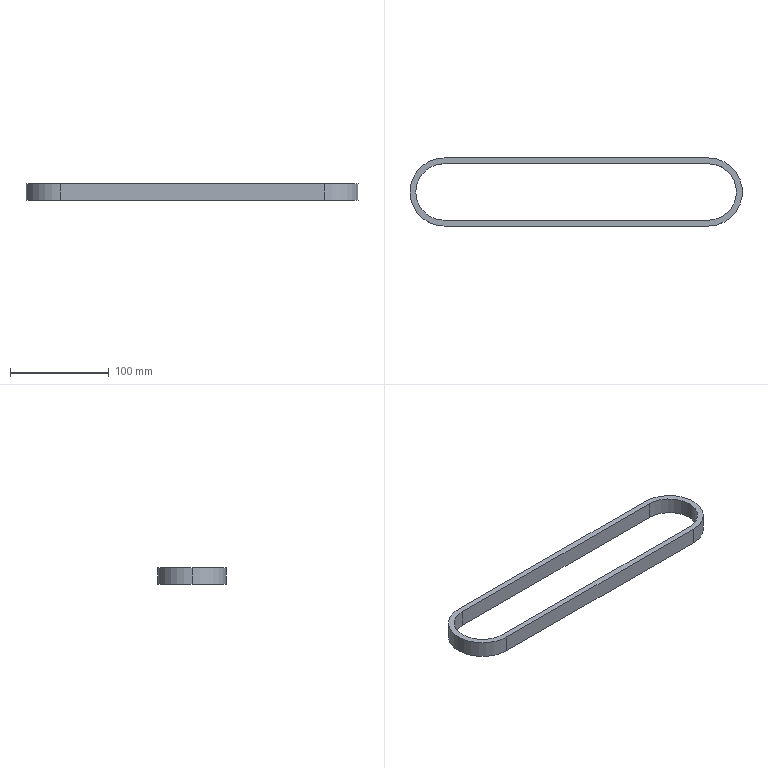Part | SolidWorks | features BaseBody 1 | 1 solid | 12 faces | box 335.87 x 68.87 x 17 mm | volume 73402 mm3 | cylinder 6 | plane 6 | commonest cylinder face diameters 57.07 x3 68.87 x3
STEP:
#1=CARTESIAN_POINT('',(0.,28.535,17.));
#2=VERTEX_POINT('',#1);
#3=CARTESIAN_POINT('',(-28.535,0.,17.));
#4=VERTEX_POINT('',#3);
#5=CARTESIAN_POINT('',(0.,0.,17.));
#6=DIRECTION('',(0.,0.,1.));
#7=DIRECTION('',(1.,0.,0.));
#8=AXIS2_PLACEMENT_3D('',#5,#6,#7);
#9=CIRCLE('',#8,28.535);
#10=EDGE_CURVE('',#2,#4,#9,.T.);
#11=ORIENTED_EDGE('',*,*,#10,.T.);
#12=CARTESIAN_POINT('',(-28.535,0.,0.));
#13=VERTEX_POINT('',#12);
#14=CARTESIAN_POINT('',(-28.535,0.,17.));
#15=DIRECTION('',(0.,0.,-1.));
#16=VECTOR('',#15,1000.);
#17=LINE('',#14,#16);
#18=EDGE_CURVE('',#4,#13,#17,.T.);
#19=ORIENTED_EDGE('',*,*,#18,.T.);
#20=CARTESIAN_POINT('',(0.,28.535,0.));
#21=VERTEX_POINT('',#20);
#22=CARTESIAN_POINT('',(0.,0.,0.));
#23=DIRECTION('',(0.,0.,1.));
#24=DIRECTION('',(1.,0.,0.));
#25=AXIS2_PLACEMENT_3D('',#22,#23,#24);
#26=CIRCLE('',#25,28.535);
#27=EDGE_CURVE('',#21,#13,#26,.T.);
#28=ORIENTED_EDGE('',*,*,#27,.F.);
#29=CARTESIAN_POINT('',(0.,28.535,17.));
#30=DIRECTION('',(0.,0.,-1.));
#31=VECTOR('',#30,1000.);
#32=LINE('',#29,#31);
#33=EDGE_CURVE('',#2,#21,#32,.T.);
#34=ORIENTED_EDGE('',*,*,#33,.F.);
#35=EDGE_LOOP('',(#11,#19,#28,#34));
#36=FACE_OUTER_BOUND('',#35,.T.);
#37=CARTESIAN_POINT('',(0.,0.,17.));
#38=DIRECTION('',(0.,0.,-1.));
#39=DIRECTION('',(-1.,0.,0.));
#40=AXIS2_PLACEMENT_3D('',#37,#38,#39);
#41=CYLINDRICAL_SURFACE('',#40,28.535);
#42=ADVANCED_FACE('',(#36),#41,.F.);
#43=CARTESIAN_POINT('',(-34.435,0.,17.));
#44=VERTEX_POINT('',#43);
#45=CARTESIAN_POINT('',(0.,-34.435,17.));
#46=VERTEX_POINT('',#45);
#47=CARTESIAN_POINT('',(0.,0.,17.));
#48=DIRECTION('',(0.,0.,1.));
#49=DIRECTION('',(1.,0.,0.));
#50=AXIS2_PLACEMENT_3D('',#47,#48,#49);
#51=CIRCLE('',#50,34.435);
#52=EDGE_CURVE('',#44,#46,#51,.T.);
#53=ORIENTED_EDGE('',*,*,#52,.F.);
#54=CARTESIAN_POINT('',(-34.435,0.,0.));
#55=VERTEX_POINT('',#54);
#56=CARTESIAN_POINT('',(-34.435,0.,17.));
#57=DIRECTION('',(0.,0.,-1.));
#58=VECTOR('',#57,1000.);
#59=LINE('',#56,#58);
#60=EDGE_CURVE('',#44,#55,#59,.T.);
#61=ORIENTED_EDGE('',*,*,#60,.T.);
#62=CARTESIAN_POINT('',(0.,-34.435,0.));
#63=VERTEX_POINT('',#62);
#64=CARTESIAN_POINT('',(0.,0.,0.));
#65=DIRECTION('',(0.,0.,1.));
#66=DIRECTION('',(1.,0.,0.));
#67=AXIS2_PLACEMENT_3D('',#64,#65,#66);
#68=CIRCLE('',#67,34.435);
#69=EDGE_CURVE('',#55,#63,#68,.T.);
#70=ORIENTED_EDGE('',*,*,#69,.T.);
#71=CARTESIAN_POINT('',(0.,-34.435,17.));
#72=DIRECTION('',(0.,0.,-1.));
#73=VECTOR('',#72,1000.);
#74=LINE('',#71,#73);
#75=EDGE_CURVE('',#46,#63,#74,.T.);
#76=ORIENTED_EDGE('',*,*,#75,.F.);
#77=EDGE_LOOP('',(#53,#61,#70,#76));
#78=FACE_OUTER_BOUND('',#77,.T.);
#79=CARTESIAN_POINT('',(0.,0.,17.));
#80=DIRECTION('',(0.,0.,-1.));
#81=DIRECTION('',(-1.,0.,0.));
#82=AXIS2_PLACEMENT_3D('',#79,#80,#81);
#83=CYLINDRICAL_SURFACE('',#82,34.435);
#84=ADVANCED_FACE('',(#78),#83,.T.);
#85=CARTESIAN_POINT('',(0.,34.435,17.));
#86=VERTEX_POINT('',#85);
#87=CARTESIAN_POINT('',(0.,0.,17.));
#88=DIRECTION('',(0.,0.,1.));
#89=DIRECTION('',(1.,0.,0.));
#90=AXIS2_PLACEMENT_3D('',#87,#88,#89);
#91=CIRCLE('',#90,34.435);
#92=EDGE_CURVE('',#86,#44,#91,.T.);
#93=ORIENTED_EDGE('',*,*,#92,.T.);
#94=ORIENTED_EDGE('',*,*,#52,.T.);
#95=CARTESIAN_POINT('',(267.,-34.435,17.));
#96=VERTEX_POINT('',#95);
#97=CARTESIAN_POINT('',(0.,-34.435,17.));
#98=DIRECTION('',(1.,0.,0.));
#99=VECTOR('',#98,1000.);
#100=LINE('',#97,#99);
#101=EDGE_CURVE('',#46,#96,#100,.T.);
#102=ORIENTED_EDGE('',*,*,#101,.T.);
#103=CARTESIAN_POINT('',(267.,34.435,17.));
#104=VERTEX_POINT('',#103);
#105=CARTESIAN_POINT('',(267.,0.,17.));
#106=DIRECTION('',(0.,0.,1.));
#107=DIRECTION('',(1.,0.,0.));
#108=AXIS2_PLACEMENT_3D('',#105,#106,#107);
#109=CIRCLE('',#108,34.435);
#110=EDGE_CURVE('',#96,#104,#109,.T.);
#111=ORIENTED_EDGE('',*,*,#110,.T.);
#112=CARTESIAN_POINT('',(0.,34.435,17.));
#113=DIRECTION('',(-1.,0.,0.));
#114=VECTOR('',#113,1000.);
#115=LINE('',#112,#114);
#116=EDGE_CURVE('',#104,#86,#115,.T.);
#117=ORIENTED_EDGE('',*,*,#116,.T.);
#118=EDGE_LOOP('',(#93,#94,#102,#111,#117));
#119=FACE_OUTER_BOUND('',#118,.T.);
#120=CARTESIAN_POINT('',(0.,-28.535,17.));
#121=VERTEX_POINT('',#120);
#122=CARTESIAN_POINT('',(267.,-28.535,17.));
#123=VERTEX_POINT('',#122);
#124=CARTESIAN_POINT('',(0.,-28.535,17.));
#125=DIRECTION('',(1.,0.,0.));
#126=VECTOR('',#125,1000.);
#127=LINE('',#124,#126);
#128=EDGE_CURVE('',#121,#123,#127,.T.);
#129=ORIENTED_EDGE('',*,*,#128,.F.);
#130=CARTESIAN_POINT('',(0.,0.,17.));
#131=DIRECTION('',(0.,0.,1.));
#132=DIRECTION('',(1.,0.,0.));
#133=AXIS2_PLACEMENT_3D('',#130,#131,#132);
#134=CIRCLE('',#133,28.535);
#135=EDGE_CURVE('',#4,#121,#134,.T.);
#136=ORIENTED_EDGE('',*,*,#135,.F.);
#137=ORIENTED_EDGE('',*,*,#10,.F.);
#138=CARTESIAN_POINT('',(267.,28.535,17.));
#139=VERTEX_POINT('',#138);
#140=CARTESIAN_POINT('',(0.,28.535,17.));
#141=DIRECTION('',(-1.,0.,0.));
#142=VECTOR('',#141,1000.);
#143=LINE('',#140,#142);
#144=EDGE_CURVE('',#139,#2,#143,.T.);
#145=ORIENTED_EDGE('',*,*,#144,.F.);
#146=CARTESIAN_POINT('',(267.,0.,17.));
#147=DIRECTION('',(0.,0.,1.));
#148=DIRECTION('',(1.,0.,0.));
#149=AXIS2_PLACEMENT_3D('',#146,#147,#148);
#150=CIRCLE('',#149,28.535);
#151=EDGE_CURVE('',#123,#139,#150,.T.);
#152=ORIENTED_EDGE('',*,*,#151,.F.);
#153=EDGE_LOOP('',(#129,#136,#137,#145,#152));
#154=FACE_BOUND('',#153,.T.);
#155=CARTESIAN_POINT('',(0.,0.,17.));
#156=DIRECTION('',(0.,0.,1.));
#157=DIRECTION('',(1.,0.,0.));
#158=AXIS2_PLACEMENT_3D('',#155,#156,#157);
#159=PLANE('',#158);
#160=ADVANCED_FACE('',(#119,#154),#159,.T.);
#161=CARTESIAN_POINT('',(0.,34.435,0.));
#162=VERTEX_POINT('',#161);
#163=CARTESIAN_POINT('',(0.,0.,0.));
#164=DIRECTION('',(0.,0.,1.));
#165=DIRECTION('',(1.,0.,0.));
#166=AXIS2_PLACEMENT_3D('',#163,#164,#165);
#167=CIRCLE('',#166,34.435);
#168=EDGE_CURVE('',#162,#55,#167,.T.);
#169=ORIENTED_EDGE('',*,*,#168,.F.);
#170=CARTESIAN_POINT('',(267.,34.435,0.));
#171=VERTEX_POINT('',#170);
#172=CARTESIAN_POINT('',(0.,34.435,0.));
#173=DIRECTION('',(-1.,0.,0.));
#174=VECTOR('',#173,1000.);
#175=LINE('',#172,#174);
#176=EDGE_CURVE('',#171,#162,#175,.T.);
#177=ORIENTED_EDGE('',*,*,#176,.F.);
#178=CARTESIAN_POINT('',(267.,-34.435,0.));
#179=VERTEX_POINT('',#178);
#180=CARTESIAN_POINT('',(267.,0.,0.));
#181=DIRECTION('',(0.,0.,1.));
#182=DIRECTION('',(1.,0.,0.));
#183=AXIS2_PLACEMENT_3D('',#180,#181,#182);
#184=CIRCLE('',#183,34.435);
#185=EDGE_CURVE('',#179,#171,#184,.T.);
#186=ORIENTED_EDGE('',*,*,#185,.F.);
#187=CARTESIAN_POINT('',(0.,-34.435,0.));
#188=DIRECTION('',(1.,0.,0.));
#189=VECTOR('',#188,1000.);
#190=LINE('',#187,#189);
#191=EDGE_CURVE('',#63,#179,#190,.T.);
#192=ORIENTED_EDGE('',*,*,#191,.F.);
#193=ORIENTED_EDGE('',*,*,#69,.F.);
#194=EDGE_LOOP('',(#169,#177,#186,#192,#193));
#195=FACE_OUTER_BOUND('',#194,.T.);
#196=ORIENTED_EDGE('',*,*,#27,.T.);
#197=CARTESIAN_POINT('',(0.,-28.535,0.));
#198=VERTEX_POINT('',#197);
#199=CARTESIAN_POINT('',(0.,0.,0.));
#200=DIRECTION('',(0.,0.,1.));
#201=DIRECTION('',(1.,0.,0.));
#202=AXIS2_PLACEMENT_3D('',#199,#200,#201);
#203=CIRCLE('',#202,28.535);
#204=EDGE_CURVE('',#13,#198,#203,.T.);
#205=ORIENTED_EDGE('',*,*,#204,.T.);
#206=CARTESIAN_POINT('',(267.,-28.535,0.));
#207=VERTEX_POINT('',#206);
#208=CARTESIAN_POINT('',(0.,-28.535,0.));
#209=DIRECTION('',(1.,0.,0.));
#210=VECTOR('',#209,1000.);
#211=LINE('',#208,#210);
#212=EDGE_CURVE('',#198,#207,#211,.T.);
#213=ORIENTED_EDGE('',*,*,#212,.T.);
#214=CARTESIAN_POINT('',(267.,28.535,0.));
#215=VERTEX_POINT('',#214);
#216=CARTESIAN_POINT('',(267.,0.,0.));
#217=DIRECTION('',(0.,0.,1.));
#218=DIRECTION('',(1.,0.,0.));
#219=AXIS2_PLACEMENT_3D('',#216,#217,#218);
#220=CIRCLE('',#219,28.535);
#221=EDGE_CURVE('',#207,#215,#220,.T.);
#222=ORIENTED_EDGE('',*,*,#221,.T.);
#223=CARTESIAN_POINT('',(0.,28.535,0.));
#224=DIRECTION('',(-1.,0.,0.));
#225=VECTOR('',#224,1000.);
#226=LINE('',#223,#225);
#227=EDGE_CURVE('',#215,#21,#226,.T.);
#228=ORIENTED_EDGE('',*,*,#227,.T.);
#229=EDGE_LOOP('',(#196,#205,#213,#222,#228));
#230=FACE_BOUND('',#229,.T.);
#231=CARTESIAN_POINT('',(0.,0.,0.));
#232=DIRECTION('',(0.,0.,1.));
#233=DIRECTION('',(1.,0.,0.));
#234=AXIS2_PLACEMENT_3D('',#231,#232,#233);
#235=PLANE('',#234);
#236=ADVANCED_FACE('',(#195,#230),#235,.F.);
#237=ORIENTED_EDGE('',*,*,#60,.F.);
#238=ORIENTED_EDGE('',*,*,#92,.F.);
#239=CARTESIAN_POINT('',(0.,34.435,17.));
#240=DIRECTION('',(0.,0.,-1.));
#241=VECTOR('',#240,1000.);
#242=LINE('',#239,#241);
#243=EDGE_CURVE('',#86,#162,#242,.T.);
#244=ORIENTED_EDGE('',*,*,#243,.T.);
#245=ORIENTED_EDGE('',*,*,#168,.T.);
#246=EDGE_LOOP('',(#237,#238,#244,#245));
#247=FACE_OUTER_BOUND('',#246,.T.);
#248=CARTESIAN_POINT('',(0.,0.,17.));
#249=DIRECTION('',(0.,0.,-1.));
#250=DIRECTION('',(-1.,0.,0.));
#251=AXIS2_PLACEMENT_3D('',#248,#249,#250);
#252=CYLINDRICAL_SURFACE('',#251,34.435);
#253=ADVANCED_FACE('',(#247),#252,.T.);
#254=ORIENTED_EDGE('',*,*,#191,.T.);
#255=CARTESIAN_POINT('',(267.,-34.435,17.));
#256=DIRECTION('',(0.,0.,-1.));
#257=VECTOR('',#256,1000.);
#258=LINE('',#255,#257);
#259=EDGE_CURVE('',#96,#179,#258,.T.);
#260=ORIENTED_EDGE('',*,*,#259,.F.);
#261=ORIENTED_EDGE('',*,*,#101,.F.);
#262=ORIENTED_EDGE('',*,*,#75,.T.);
#263=EDGE_LOOP('',(#254,#260,#261,#262));
#264=FACE_OUTER_BOUND('',#263,.T.);
#265=CARTESIAN_POINT('',(0.,-34.435,17.));
#266=DIRECTION('',(0.,1.,0.));
#267=DIRECTION('',(0.,0.,1.));
#268=AXIS2_PLACEMENT_3D('',#265,#266,#267);
#269=PLANE('',#268);
#270=ADVANCED_FACE('',(#264),#269,.F.);
#271=ORIENTED_EDGE('',*,*,#185,.T.);
#272=CARTESIAN_POINT('',(267.,34.435,17.));
#273=DIRECTION('',(0.,0.,-1.));
#274=VECTOR('',#273,1000.);
#275=LINE('',#272,#274);
#276=EDGE_CURVE('',#104,#171,#275,.T.);
#277=ORIENTED_EDGE('',*,*,#276,.F.);
#278=ORIENTED_EDGE('',*,*,#110,.F.);
#279=ORIENTED_EDGE('',*,*,#259,.T.);
#280=EDGE_LOOP('',(#271,#277,#278,#279));
#281=FACE_OUTER_BOUND('',#280,.T.);
#282=CARTESIAN_POINT('',(267.,0.,17.));
#283=DIRECTION('',(0.,0.,-1.));
#284=DIRECTION('',(-1.,0.,0.));
#285=AXIS2_PLACEMENT_3D('',#282,#283,#284);
#286=CYLINDRICAL_SURFACE('',#285,34.435);
#287=ADVANCED_FACE('',(#281),#286,.T.);
#288=ORIENTED_EDGE('',*,*,#176,.T.);
#289=ORIENTED_EDGE('',*,*,#243,.F.);
#290=ORIENTED_EDGE('',*,*,#116,.F.);
#291=ORIENTED_EDGE('',*,*,#276,.T.);
#292=EDGE_LOOP('',(#288,#289,#290,#291));
#293=FACE_OUTER_BOUND('',#292,.T.);
#294=CARTESIAN_POINT('',(0.,34.435,17.));
#295=DIRECTION('',(0.,-1.,0.));
#296=DIRECTION('',(0.,0.,-1.));
#297=AXIS2_PLACEMENT_3D('',#294,#295,#296);
#298=PLANE('',#297);
#299=ADVANCED_FACE('',(#293),#298,.F.);
#300=ORIENTED_EDGE('',*,*,#18,.F.);
#301=ORIENTED_EDGE('',*,*,#135,.T.);
#302=CARTESIAN_POINT('',(0.,-28.535,17.));
#303=DIRECTION('',(0.,0.,-1.));
#304=VECTOR('',#303,1000.);
#305=LINE('',#302,#304);
#306=EDGE_CURVE('',#121,#198,#305,.T.);
#307=ORIENTED_EDGE('',*,*,#306,.T.);
#308=ORIENTED_EDGE('',*,*,#204,.F.);
#309=EDGE_LOOP('',(#300,#301,#307,#308));
#310=FACE_OUTER_BOUND('',#309,.T.);
#311=CARTESIAN_POINT('',(0.,0.,17.));
#312=DIRECTION('',(0.,0.,-1.));
#313=DIRECTION('',(-1.,0.,0.));
#314=AXIS2_PLACEMENT_3D('',#311,#312,#313);
#315=CYLINDRICAL_SURFACE('',#314,28.535);
#316=ADVANCED_FACE('',(#310),#315,.F.);
#317=ORIENTED_EDGE('',*,*,#212,.F.);
#318=ORIENTED_EDGE('',*,*,#306,.F.);
#319=ORIENTED_EDGE('',*,*,#128,.T.);
#320=CARTESIAN_POINT('',(267.,-28.535,17.));
#321=DIRECTION('',(0.,0.,-1.));
#322=VECTOR('',#321,1000.);
#323=LINE('',#320,#322);
#324=EDGE_CURVE('',#123,#207,#323,.T.);
#325=ORIENTED_EDGE('',*,*,#324,.T.);
#326=EDGE_LOOP('',(#317,#318,#319,#325));
#327=FACE_OUTER_BOUND('',#326,.T.);
#328=CARTESIAN_POINT('',(0.,-28.535,17.));
#329=DIRECTION('',(0.,1.,0.));
#330=DIRECTION('',(-1.,0.,0.));
#331=AXIS2_PLACEMENT_3D('',#328,#329,#330);
#332=PLANE('',#331);
#333=ADVANCED_FACE('',(#327),#332,.T.);
#334=ORIENTED_EDGE('',*,*,#221,.F.);
#335=ORIENTED_EDGE('',*,*,#324,.F.);
#336=ORIENTED_EDGE('',*,*,#151,.T.);
#337=CARTESIAN_POINT('',(267.,28.535,17.));
#338=DIRECTION('',(0.,0.,-1.));
#339=VECTOR('',#338,1000.);
#340=LINE('',#337,#339);
#341=EDGE_CURVE('',#139,#215,#340,.T.);
#342=ORIENTED_EDGE('',*,*,#341,.T.);
#343=EDGE_LOOP('',(#334,#335,#336,#342));
#344=FACE_OUTER_BOUND('',#343,.T.);
#345=CARTESIAN_POINT('',(267.,0.,17.));
#346=DIRECTION('',(0.,0.,-1.));
#347=DIRECTION('',(-1.,0.,0.));
#348=AXIS2_PLACEMENT_3D('',#345,#346,#347);
#349=CYLINDRICAL_SURFACE('',#348,28.535);
#350=ADVANCED_FACE('',(#344),#349,.F.);
#351=ORIENTED_EDGE('',*,*,#227,.F.);
#352=ORIENTED_EDGE('',*,*,#341,.F.);
#353=ORIENTED_EDGE('',*,*,#144,.T.);
#354=ORIENTED_EDGE('',*,*,#33,.T.);
#355=EDGE_LOOP('',(#351,#352,#353,#354));
#356=FACE_OUTER_BOUND('',#355,.T.);
#357=CARTESIAN_POINT('',(0.,28.535,17.));
#358=DIRECTION('',(0.,-1.,0.));
#359=DIRECTION('',(1.,0.,0.));
#360=AXIS2_PLACEMENT_3D('',#357,#358,#359);
#361=PLANE('',#360);
#362=ADVANCED_FACE('',(#356),#361,.T.);
#363=CLOSED_SHELL('',(#42,#84,#160,#236,#253,#270,#287,#299,#316,#333,#350,#362));
#364=MANIFOLD_SOLID_BREP('',#363);
#365=CARTESIAN_POINT('',(0.,0.,0.));
#366=DIRECTION('',(0.,0.,1.));
#367=DIRECTION('',(1.,0.,0.));
#368=AXIS2_PLACEMENT_3D('',#365,#366,#367);
#369=(LENGTH_UNIT()NAMED_UNIT(*)SI_UNIT(.MILLI.,.METRE.));
#370=UNCERTAINTY_MEASURE_WITH_UNIT(LENGTH_MEASURE(0.00001),#369,'','');
#371=(NAMED_UNIT(*)PLANE_ANGLE_UNIT()SI_UNIT($,.RADIAN.));
#372=(NAMED_UNIT(*)SI_UNIT($,.STERADIAN.)SOLID_ANGLE_UNIT());
#373=(GEOMETRIC_REPRESENTATION_CONTEXT(3)GLOBAL_UNCERTAINTY_ASSIGNED_CONTEXT((#370))GLOBAL_UNIT_ASSIGNED_CONTEXT((#369,#371,#372))REPRESENTATION_CONTEXT('',''));
#374=ADVANCED_BREP_SHAPE_REPRESENTATION('',(#364,#368),#373);